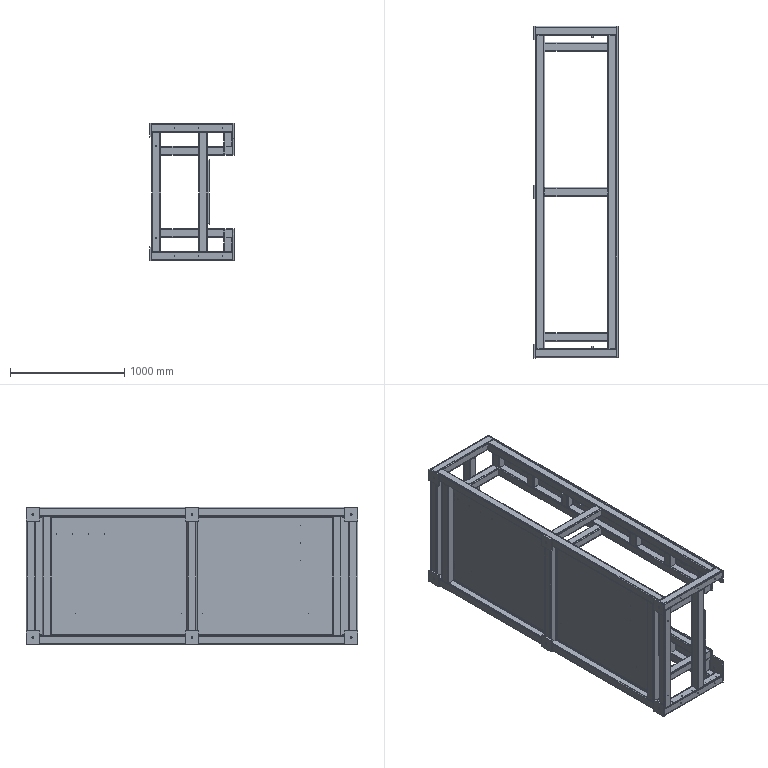Part | SolidWorks | features BaseBody 53 | 53 solids | 1606 faces | box 735 x 2900 x 1200 mm | volume 73256016 mm3 | cylinder 1012 | plane 514 | cone 64 | sphere 16 | commonest cylinder face diameters 6.8 x290 5 x180 10 x164 20 x156 3.3 x92 4.2 x68